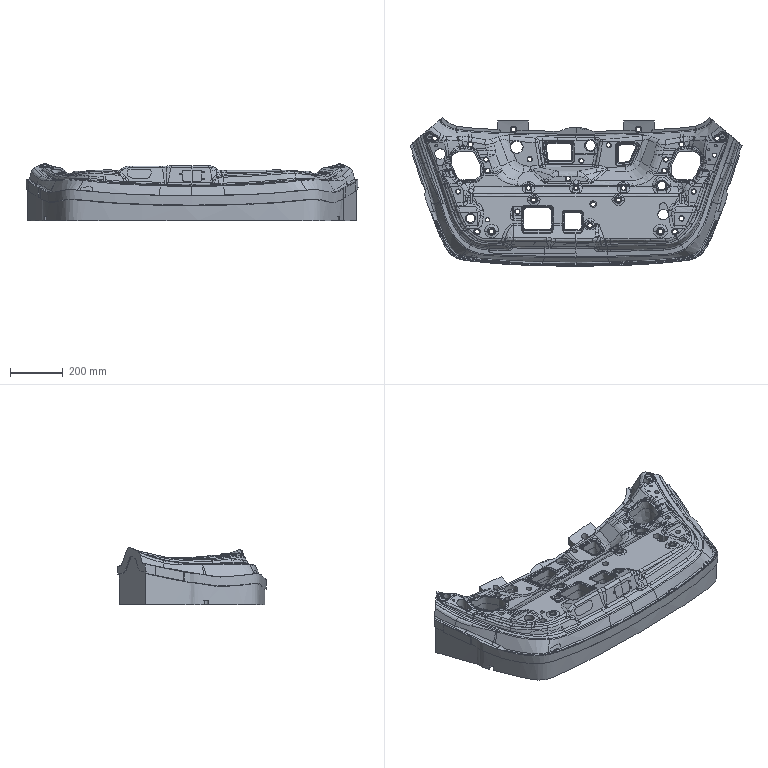Part | NX | features solid 2 | 1 solid | 1740 faces | box 1258 x 563.164 x 216.429 mm | volume 74842691 mm3 | spline 1460 | plane 150 | cylinder 130 | commonest cylinder face diameters 16 x24 20 x22 23 x22 25 x15 43 x10 17 x7